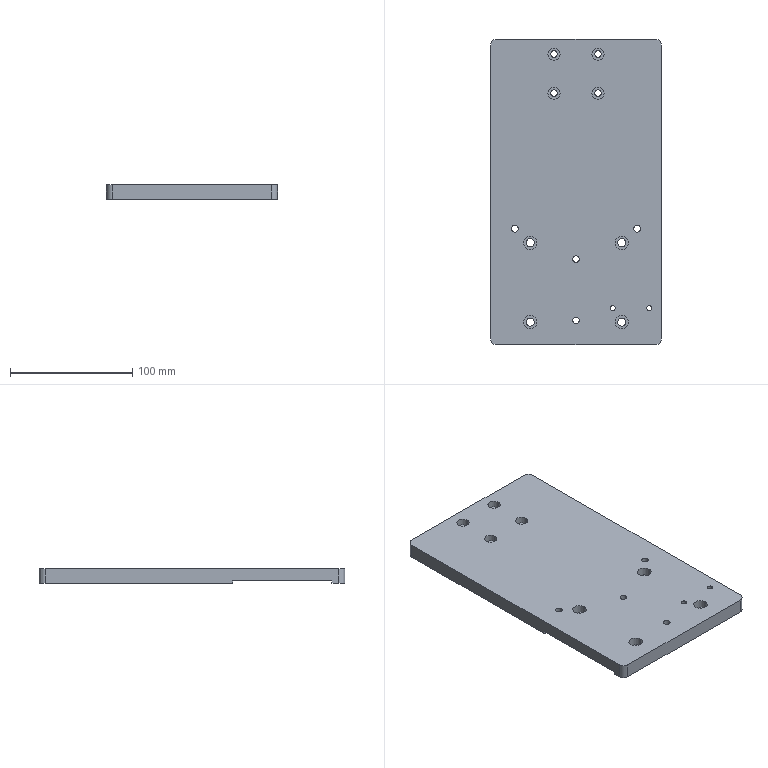Part | SolidWorks | features HoleWzd 5, Extrusion 1, Fillet 1, ICE 1 | 1 solid | 80 faces | box 140 x 250 x 12 mm | volume 389185 mm3 | cylinder 56 | plane 24 | commonest cylinder face diameters 10 x20 5.5 x16 6.6 x8 11 x8 4.2 x4